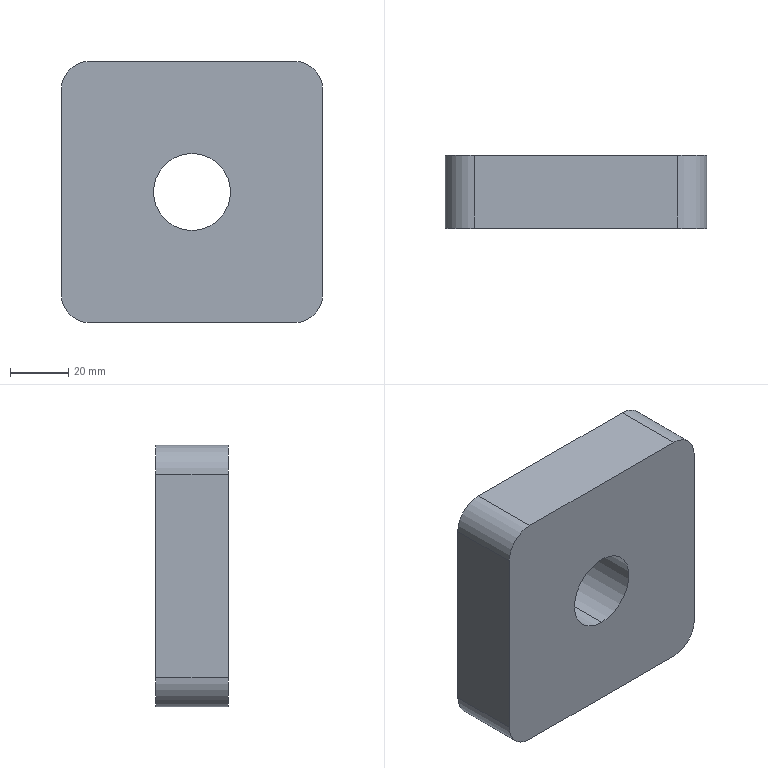Part | SolidWorks | features BaseBody 1 | 1 solid | 12 faces | box 90 x 25 x 90 mm | volume 186565 mm3 | cylinder 6 | plane 6 | commonest cylinder face diameters 20 x4 26.5 x2
STEP:
#1=CARTESIAN_POINT('',(0.,-15.,13.25));
#2=VERTEX_POINT('',#1);
#3=CARTESIAN_POINT('',(0.,-15.,-13.25));
#4=VERTEX_POINT('',#3);
#5=CARTESIAN_POINT('',(0.,-15.,0.));
#6=DIRECTION('',(0.,-1.,0.));
#7=DIRECTION('',(0.,0.,-1.));
#8=AXIS2_PLACEMENT_3D('',#5,#6,#7);
#9=CIRCLE('',#8,13.25);
#10=EDGE_CURVE('',#2,#4,#9,.T.);
#11=ORIENTED_EDGE('',*,*,#10,.T.);
#12=CARTESIAN_POINT('',(0.,10.,-13.25));
#13=VERTEX_POINT('',#12);
#14=CARTESIAN_POINT('',(0.,10.,-13.25));
#15=DIRECTION('',(0.,1.,0.));
#16=VECTOR('',#15,1000.);
#17=LINE('',#14,#16);
#18=EDGE_CURVE('',#4,#13,#17,.T.);
#19=ORIENTED_EDGE('',*,*,#18,.T.);
#20=CARTESIAN_POINT('',(0.,10.,13.25));
#21=VERTEX_POINT('',#20);
#22=CARTESIAN_POINT('',(0.,10.,0.));
#23=DIRECTION('',(0.,1.,0.));
#24=DIRECTION('',(0.,0.,1.));
#25=AXIS2_PLACEMENT_3D('',#22,#23,#24);
#26=CIRCLE('',#25,13.25);
#27=EDGE_CURVE('',#13,#21,#26,.T.);
#28=ORIENTED_EDGE('',*,*,#27,.T.);
#29=CARTESIAN_POINT('',(0.,10.,13.25));
#30=DIRECTION('',(0.,1.,0.));
#31=VECTOR('',#30,1000.);
#32=LINE('',#29,#31);
#33=EDGE_CURVE('',#2,#21,#32,.T.);
#34=ORIENTED_EDGE('',*,*,#33,.F.);
#35=EDGE_LOOP('',(#11,#19,#28,#34));
#36=FACE_OUTER_BOUND('',#35,.T.);
#37=CARTESIAN_POINT('',(0.,10.,0.));
#38=DIRECTION('',(0.,1.,0.));
#39=DIRECTION('',(0.,0.,1.));
#40=AXIS2_PLACEMENT_3D('',#37,#38,#39);
#41=CYLINDRICAL_SURFACE('',#40,13.25);
#42=ADVANCED_FACE('',(#36),#41,.F.);
#43=CARTESIAN_POINT('',(45.,10.,-35.));
#44=VERTEX_POINT('',#43);
#45=CARTESIAN_POINT('',(35.,10.,-45.));
#46=VERTEX_POINT('',#45);
#47=CARTESIAN_POINT('',(35.,10.,-35.));
#48=DIRECTION('',(0.,1.,0.));
#49=DIRECTION('',(0.,0.,1.));
#50=AXIS2_PLACEMENT_3D('',#47,#48,#49);
#51=CIRCLE('',#50,10.);
#52=EDGE_CURVE('',#44,#46,#51,.T.);
#53=ORIENTED_EDGE('',*,*,#52,.F.);
#54=CARTESIAN_POINT('',(45.,-15.,-35.));
#55=VERTEX_POINT('',#54);
#56=CARTESIAN_POINT('',(45.,15.,-35.));
#57=DIRECTION('',(0.,-1.,0.));
#58=VECTOR('',#57,1000.);
#59=LINE('',#56,#58);
#60=EDGE_CURVE('',#44,#55,#59,.T.);
#61=ORIENTED_EDGE('',*,*,#60,.T.);
#62=CARTESIAN_POINT('',(35.,-15.,-45.));
#63=VERTEX_POINT('',#62);
#64=CARTESIAN_POINT('',(35.,-15.,-35.));
#65=DIRECTION('',(0.,1.,0.));
#66=DIRECTION('',(0.,0.,-1.));
#67=AXIS2_PLACEMENT_3D('',#64,#65,#66);
#68=CIRCLE('',#67,10.);
#69=EDGE_CURVE('',#55,#63,#68,.T.);
#70=ORIENTED_EDGE('',*,*,#69,.T.);
#71=CARTESIAN_POINT('',(35.,15.,-45.));
#72=DIRECTION('',(0.,-1.,0.));
#73=VECTOR('',#72,1000.);
#74=LINE('',#71,#73);
#75=EDGE_CURVE('',#46,#63,#74,.T.);
#76=ORIENTED_EDGE('',*,*,#75,.F.);
#77=EDGE_LOOP('',(#53,#61,#70,#76));
#78=FACE_OUTER_BOUND('',#77,.T.);
#79=CARTESIAN_POINT('',(35.,15.,-35.));
#80=DIRECTION('',(0.,-1.,0.));
#81=DIRECTION('',(0.,0.,-1.));
#82=AXIS2_PLACEMENT_3D('',#79,#80,#81);
#83=CYLINDRICAL_SURFACE('',#82,10.);
#84=ADVANCED_FACE('',(#78),#83,.T.);
#85=CARTESIAN_POINT('',(-35.,10.,-45.));
#86=VERTEX_POINT('',#85);
#87=CARTESIAN_POINT('',(35.,10.,-45.));
#88=DIRECTION('',(-1.,0.,0.));
#89=VECTOR('',#88,1000.);
#90=LINE('',#87,#89);
#91=EDGE_CURVE('',#46,#86,#90,.T.);
#92=ORIENTED_EDGE('',*,*,#91,.F.);
#93=ORIENTED_EDGE('',*,*,#75,.T.);
#94=CARTESIAN_POINT('',(-35.,-15.,-45.));
#95=VERTEX_POINT('',#94);
#96=CARTESIAN_POINT('',(-35.,-15.,-45.));
#97=DIRECTION('',(-1.,0.,0.));
#98=VECTOR('',#97,1000.);
#99=LINE('',#96,#98);
#100=EDGE_CURVE('',#63,#95,#99,.T.);
#101=ORIENTED_EDGE('',*,*,#100,.T.);
#102=CARTESIAN_POINT('',(-35.,15.,-45.));
#103=DIRECTION('',(0.,-1.,0.));
#104=VECTOR('',#103,1000.);
#105=LINE('',#102,#104);
#106=EDGE_CURVE('',#86,#95,#105,.T.);
#107=ORIENTED_EDGE('',*,*,#106,.F.);
#108=EDGE_LOOP('',(#92,#93,#101,#107));
#109=FACE_OUTER_BOUND('',#108,.T.);
#110=CARTESIAN_POINT('',(-35.,15.,-45.));
#111=DIRECTION('',(0.,0.,1.));
#112=DIRECTION('',(1.,0.,0.));
#113=AXIS2_PLACEMENT_3D('',#110,#111,#112);
#114=PLANE('',#113);
#115=ADVANCED_FACE('',(#109),#114,.F.);
#116=CARTESIAN_POINT('',(-45.,10.,-35.));
#117=VERTEX_POINT('',#116);
#118=CARTESIAN_POINT('',(-35.,10.,-35.));
#119=DIRECTION('',(0.,1.,0.));
#120=DIRECTION('',(0.,0.,1.));
#121=AXIS2_PLACEMENT_3D('',#118,#119,#120);
#122=CIRCLE('',#121,10.);
#123=EDGE_CURVE('',#86,#117,#122,.T.);
#124=ORIENTED_EDGE('',*,*,#123,.F.);
#125=ORIENTED_EDGE('',*,*,#106,.T.);
#126=CARTESIAN_POINT('',(-45.,-15.,-35.));
#127=VERTEX_POINT('',#126);
#128=CARTESIAN_POINT('',(-35.,-15.,-35.));
#129=DIRECTION('',(0.,1.,0.));
#130=DIRECTION('',(0.,0.,1.));
#131=AXIS2_PLACEMENT_3D('',#128,#129,#130);
#132=CIRCLE('',#131,10.);
#133=EDGE_CURVE('',#95,#127,#132,.T.);
#134=ORIENTED_EDGE('',*,*,#133,.T.);
#135=CARTESIAN_POINT('',(-45.,15.,-35.));
#136=DIRECTION('',(0.,-1.,0.));
#137=VECTOR('',#136,1000.);
#138=LINE('',#135,#137);
#139=EDGE_CURVE('',#117,#127,#138,.T.);
#140=ORIENTED_EDGE('',*,*,#139,.F.);
#141=EDGE_LOOP('',(#124,#125,#134,#140));
#142=FACE_OUTER_BOUND('',#141,.T.);
#143=CARTESIAN_POINT('',(-35.,15.,-35.));
#144=DIRECTION('',(0.,-1.,0.));
#145=DIRECTION('',(0.,0.,-1.));
#146=AXIS2_PLACEMENT_3D('',#143,#144,#145);
#147=CYLINDRICAL_SURFACE('',#146,10.);
#148=ADVANCED_FACE('',(#142),#147,.T.);
#149=CARTESIAN_POINT('',(-45.,10.,35.));
#150=VERTEX_POINT('',#149);
#151=CARTESIAN_POINT('',(-45.,10.,-35.));
#152=DIRECTION('',(0.,0.,1.));
#153=VECTOR('',#152,1000.);
#154=LINE('',#151,#153);
#155=EDGE_CURVE('',#117,#150,#154,.T.);
#156=ORIENTED_EDGE('',*,*,#155,.F.);
#157=ORIENTED_EDGE('',*,*,#139,.T.);
#158=CARTESIAN_POINT('',(-45.,-15.,35.));
#159=VERTEX_POINT('',#158);
#160=CARTESIAN_POINT('',(-45.,-15.,-35.));
#161=DIRECTION('',(0.,0.,1.));
#162=VECTOR('',#161,1000.);
#163=LINE('',#160,#162);
#164=EDGE_CURVE('',#127,#159,#163,.T.);
#165=ORIENTED_EDGE('',*,*,#164,.T.);
#166=CARTESIAN_POINT('',(-45.,15.,35.));
#167=DIRECTION('',(0.,-1.,0.));
#168=VECTOR('',#167,1000.);
#169=LINE('',#166,#168);
#170=EDGE_CURVE('',#150,#159,#169,.T.);
#171=ORIENTED_EDGE('',*,*,#170,.F.);
#172=EDGE_LOOP('',(#156,#157,#165,#171));
#173=FACE_OUTER_BOUND('',#172,.T.);
#174=CARTESIAN_POINT('',(-45.,15.,-35.));
#175=DIRECTION('',(1.,0.,0.));
#176=DIRECTION('',(0.,0.,-1.));
#177=AXIS2_PLACEMENT_3D('',#174,#175,#176);
#178=PLANE('',#177);
#179=ADVANCED_FACE('',(#173),#178,.F.);
#180=CARTESIAN_POINT('',(-35.,10.,45.));
#181=VERTEX_POINT('',#180);
#182=CARTESIAN_POINT('',(-35.,10.,35.));
#183=DIRECTION('',(0.,1.,0.));
#184=DIRECTION('',(0.,0.,1.));
#185=AXIS2_PLACEMENT_3D('',#182,#183,#184);
#186=CIRCLE('',#185,10.);
#187=EDGE_CURVE('',#150,#181,#186,.T.);
#188=ORIENTED_EDGE('',*,*,#187,.F.);
#189=ORIENTED_EDGE('',*,*,#170,.T.);
#190=CARTESIAN_POINT('',(-35.,-15.,45.));
#191=VERTEX_POINT('',#190);
#192=CARTESIAN_POINT('',(-35.,-15.,35.));
#193=DIRECTION('',(0.,1.,0.));
#194=DIRECTION('',(0.,0.,1.));
#195=AXIS2_PLACEMENT_3D('',#192,#193,#194);
#196=CIRCLE('',#195,10.);
#197=EDGE_CURVE('',#159,#191,#196,.T.);
#198=ORIENTED_EDGE('',*,*,#197,.T.);
#199=CARTESIAN_POINT('',(-35.,15.,45.));
#200=DIRECTION('',(0.,-1.,0.));
#201=VECTOR('',#200,1000.);
#202=LINE('',#199,#201);
#203=EDGE_CURVE('',#181,#191,#202,.T.);
#204=ORIENTED_EDGE('',*,*,#203,.F.);
#205=EDGE_LOOP('',(#188,#189,#198,#204));
#206=FACE_OUTER_BOUND('',#205,.T.);
#207=CARTESIAN_POINT('',(-35.,15.,35.));
#208=DIRECTION('',(0.,-1.,0.));
#209=DIRECTION('',(0.,0.,-1.));
#210=AXIS2_PLACEMENT_3D('',#207,#208,#209);
#211=CYLINDRICAL_SURFACE('',#210,10.);
#212=ADVANCED_FACE('',(#206),#211,.T.);
#213=CARTESIAN_POINT('',(35.,10.,45.));
#214=VERTEX_POINT('',#213);
#215=CARTESIAN_POINT('',(-35.,10.,45.));
#216=DIRECTION('',(1.,0.,0.));
#217=VECTOR('',#216,1000.);
#218=LINE('',#215,#217);
#219=EDGE_CURVE('',#181,#214,#218,.T.);
#220=ORIENTED_EDGE('',*,*,#219,.F.);
#221=ORIENTED_EDGE('',*,*,#203,.T.);
#222=CARTESIAN_POINT('',(35.,-15.,45.));
#223=VERTEX_POINT('',#222);
#224=CARTESIAN_POINT('',(-35.,-15.,45.));
#225=DIRECTION('',(1.,0.,0.));
#226=VECTOR('',#225,1000.);
#227=LINE('',#224,#226);
#228=EDGE_CURVE('',#191,#223,#227,.T.);
#229=ORIENTED_EDGE('',*,*,#228,.T.);
#230=CARTESIAN_POINT('',(35.,15.,45.));
#231=DIRECTION('',(0.,-1.,0.));
#232=VECTOR('',#231,1000.);
#233=LINE('',#230,#232);
#234=EDGE_CURVE('',#214,#223,#233,.T.);
#235=ORIENTED_EDGE('',*,*,#234,.F.);
#236=EDGE_LOOP('',(#220,#221,#229,#235));
#237=FACE_OUTER_BOUND('',#236,.T.);
#238=CARTESIAN_POINT('',(-35.,15.,45.));
#239=DIRECTION('',(0.,0.,-1.));
#240=DIRECTION('',(-1.,0.,0.));
#241=AXIS2_PLACEMENT_3D('',#238,#239,#240);
#242=PLANE('',#241);
#243=ADVANCED_FACE('',(#237),#242,.F.);
#244=CARTESIAN_POINT('',(45.,10.,35.));
#245=VERTEX_POINT('',#244);
#246=CARTESIAN_POINT('',(35.,10.,35.));
#247=DIRECTION('',(0.,1.,0.));
#248=DIRECTION('',(0.,0.,1.));
#249=AXIS2_PLACEMENT_3D('',#246,#247,#248);
#250=CIRCLE('',#249,10.);
#251=EDGE_CURVE('',#214,#245,#250,.T.);
#252=ORIENTED_EDGE('',*,*,#251,.F.);
#253=ORIENTED_EDGE('',*,*,#234,.T.);
#254=CARTESIAN_POINT('',(45.,-15.,35.));
#255=VERTEX_POINT('',#254);
#256=CARTESIAN_POINT('',(35.,-15.,35.));
#257=DIRECTION('',(0.,1.,0.));
#258=DIRECTION('',(0.,0.,1.));
#259=AXIS2_PLACEMENT_3D('',#256,#257,#258);
#260=CIRCLE('',#259,10.);
#261=EDGE_CURVE('',#223,#255,#260,.T.);
#262=ORIENTED_EDGE('',*,*,#261,.T.);
#263=CARTESIAN_POINT('',(45.,15.,35.));
#264=DIRECTION('',(0.,-1.,0.));
#265=VECTOR('',#264,1000.);
#266=LINE('',#263,#265);
#267=EDGE_CURVE('',#245,#255,#266,.T.);
#268=ORIENTED_EDGE('',*,*,#267,.F.);
#269=EDGE_LOOP('',(#252,#253,#262,#268));
#270=FACE_OUTER_BOUND('',#269,.T.);
#271=CARTESIAN_POINT('',(35.,15.,35.));
#272=DIRECTION('',(0.,-1.,0.));
#273=DIRECTION('',(0.,0.,-1.));
#274=AXIS2_PLACEMENT_3D('',#271,#272,#273);
#275=CYLINDRICAL_SURFACE('',#274,10.);
#276=ADVANCED_FACE('',(#270),#275,.T.);
#277=CARTESIAN_POINT('',(45.,10.,35.));
#278=DIRECTION('',(0.,0.,-1.));
#279=VECTOR('',#278,1000.);
#280=LINE('',#277,#279);
#281=EDGE_CURVE('',#245,#44,#280,.T.);
#282=ORIENTED_EDGE('',*,*,#281,.F.);
#283=ORIENTED_EDGE('',*,*,#267,.T.);
#284=CARTESIAN_POINT('',(45.,-15.,-35.));
#285=DIRECTION('',(0.,0.,-1.));
#286=VECTOR('',#285,1000.);
#287=LINE('',#284,#286);
#288=EDGE_CURVE('',#255,#55,#287,.T.);
#289=ORIENTED_EDGE('',*,*,#288,.T.);
#290=ORIENTED_EDGE('',*,*,#60,.F.);
#291=EDGE_LOOP('',(#282,#283,#289,#290));
#292=FACE_OUTER_BOUND('',#291,.T.);
#293=CARTESIAN_POINT('',(45.,15.,-35.));
#294=DIRECTION('',(-1.,0.,0.));
#295=DIRECTION('',(0.,0.,1.));
#296=AXIS2_PLACEMENT_3D('',#293,#294,#295);
#297=PLANE('',#296);
#298=ADVANCED_FACE('',(#292),#297,.F.);
#299=ORIENTED_EDGE('',*,*,#10,.F.);
#300=CARTESIAN_POINT('',(0.,-15.,0.));
#301=DIRECTION('',(0.,-1.,0.));
#302=DIRECTION('',(0.,0.,-1.));
#303=AXIS2_PLACEMENT_3D('',#300,#301,#302);
#304=CIRCLE('',#303,13.25);
#305=EDGE_CURVE('',#4,#2,#304,.T.);
#306=ORIENTED_EDGE('',*,*,#305,.F.);
#307=EDGE_LOOP('',(#299,#306));
#308=FACE_BOUND('',#307,.T.);
#309=ORIENTED_EDGE('',*,*,#69,.F.);
#310=ORIENTED_EDGE('',*,*,#288,.F.);
#311=ORIENTED_EDGE('',*,*,#261,.F.);
#312=ORIENTED_EDGE('',*,*,#228,.F.);
#313=ORIENTED_EDGE('',*,*,#197,.F.);
#314=ORIENTED_EDGE('',*,*,#164,.F.);
#315=ORIENTED_EDGE('',*,*,#133,.F.);
#316=ORIENTED_EDGE('',*,*,#100,.F.);
#317=EDGE_LOOP('',(#309,#310,#311,#312,#313,#314,#315,#316));
#318=FACE_OUTER_BOUND('',#317,.T.);
#319=CARTESIAN_POINT('',(35.,-15.,-35.));
#320=DIRECTION('',(0.,-1.,0.));
#321=DIRECTION('',(0.,0.,-1.));
#322=AXIS2_PLACEMENT_3D('',#319,#320,#321);
#323=PLANE('',#322);
#324=ADVANCED_FACE('',(#308,#318),#323,.T.);
#325=CARTESIAN_POINT('',(0.,10.,0.));
#326=DIRECTION('',(0.,1.,0.));
#327=DIRECTION('',(0.,0.,1.));
#328=AXIS2_PLACEMENT_3D('',#325,#326,#327);
#329=CIRCLE('',#328,13.25);
#330=EDGE_CURVE('',#21,#13,#329,.T.);
#331=ORIENTED_EDGE('',*,*,#330,.F.);
#332=ORIENTED_EDGE('',*,*,#27,.F.);
#333=EDGE_LOOP('',(#331,#332));
#334=FACE_BOUND('',#333,.T.);
#335=ORIENTED_EDGE('',*,*,#52,.T.);
#336=ORIENTED_EDGE('',*,*,#91,.T.);
#337=ORIENTED_EDGE('',*,*,#123,.T.);
#338=ORIENTED_EDGE('',*,*,#155,.T.);
#339=ORIENTED_EDGE('',*,*,#187,.T.);
#340=ORIENTED_EDGE('',*,*,#219,.T.);
#341=ORIENTED_EDGE('',*,*,#251,.T.);
#342=ORIENTED_EDGE('',*,*,#281,.T.);
#343=EDGE_LOOP('',(#335,#336,#337,#338,#339,#340,#341,#342));
#344=FACE_OUTER_BOUND('',#343,.T.);
#345=CARTESIAN_POINT('',(35.,10.,-35.));
#346=DIRECTION('',(0.,1.,0.));
#347=DIRECTION('',(0.,0.,1.));
#348=AXIS2_PLACEMENT_3D('',#345,#346,#347);
#349=PLANE('',#348);
#350=ADVANCED_FACE('',(#334,#344),#349,.T.);
#351=ORIENTED_EDGE('',*,*,#18,.F.);
#352=ORIENTED_EDGE('',*,*,#305,.T.);
#353=ORIENTED_EDGE('',*,*,#33,.T.);
#354=ORIENTED_EDGE('',*,*,#330,.T.);
#355=EDGE_LOOP('',(#351,#352,#353,#354));
#356=FACE_OUTER_BOUND('',#355,.T.);
#357=CARTESIAN_POINT('',(0.,10.,0.));
#358=DIRECTION('',(0.,1.,0.));
#359=DIRECTION('',(0.,0.,1.));
#360=AXIS2_PLACEMENT_3D('',#357,#358,#359);
#361=CYLINDRICAL_SURFACE('',#360,13.25);
#362=ADVANCED_FACE('',(#356),#361,.F.);
#363=CLOSED_SHELL('',(#42,#84,#115,#148,#179,#212,#243,#276,#298,#324,#350,#362));
#364=MANIFOLD_SOLID_BREP('',#363);
#365=CARTESIAN_POINT('',(0.,0.,0.));
#366=DIRECTION('',(0.,0.,1.));
#367=DIRECTION('',(1.,0.,0.));
#368=AXIS2_PLACEMENT_3D('',#365,#366,#367);
#369=(LENGTH_UNIT()NAMED_UNIT(*)SI_UNIT(.MILLI.,.METRE.));
#370=UNCERTAINTY_MEASURE_WITH_UNIT(LENGTH_MEASURE(0.00001),#369,'','');
#371=(NAMED_UNIT(*)PLANE_ANGLE_UNIT()SI_UNIT($,.RADIAN.));
#372=(NAMED_UNIT(*)SI_UNIT($,.STERADIAN.)SOLID_ANGLE_UNIT());
#373=(GEOMETRIC_REPRESENTATION_CONTEXT(3)GLOBAL_UNCERTAINTY_ASSIGNED_CONTEXT((#370))GLOBAL_UNIT_ASSIGNED_CONTEXT((#369,#371,#372))REPRESENTATION_CONTEXT('',''));
#374=ADVANCED_BREP_SHAPE_REPRESENTATION('',(#364,#368),#373);